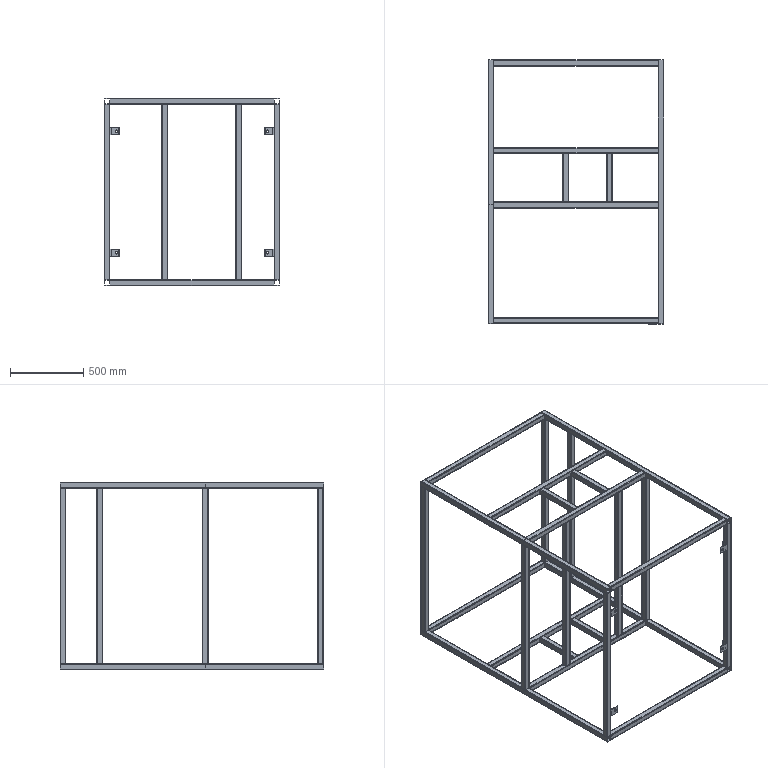Part | SolidWorks | features ReferencePattern 2, AEMSimFeature 1, LocalLPattern 1 | 31 solids | 538 faces | box 1200 x 1802 x 1280 mm | volume 10178474 mm3 | plane 302 | cylinder 236 | commonest cylinder face diameters 4.6 x108 9.2 x108 3.333 x8 17 x8 14 x4